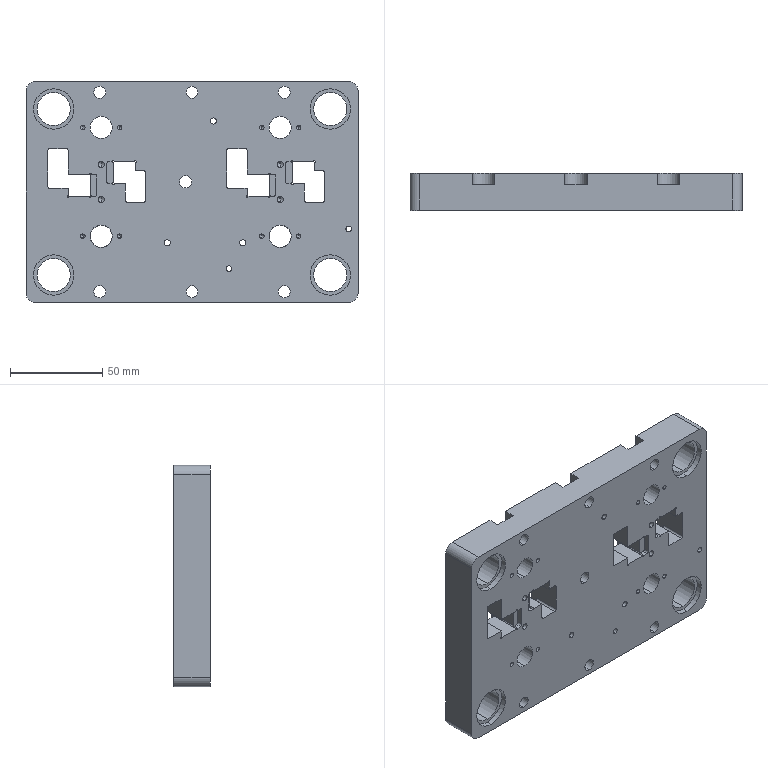Part | STEP file | 03-01 trimming base die | 1 solid | 512 faces | box 180 x 20 x 120 mm | volume 352918 mm3 | plane 224 | cylinder 203 | cone 80 | spline 5 | commonest cylinder face diameters 2 x64 2.5 x24 1 x18 12 x17 3.3 x14 6.5 x12